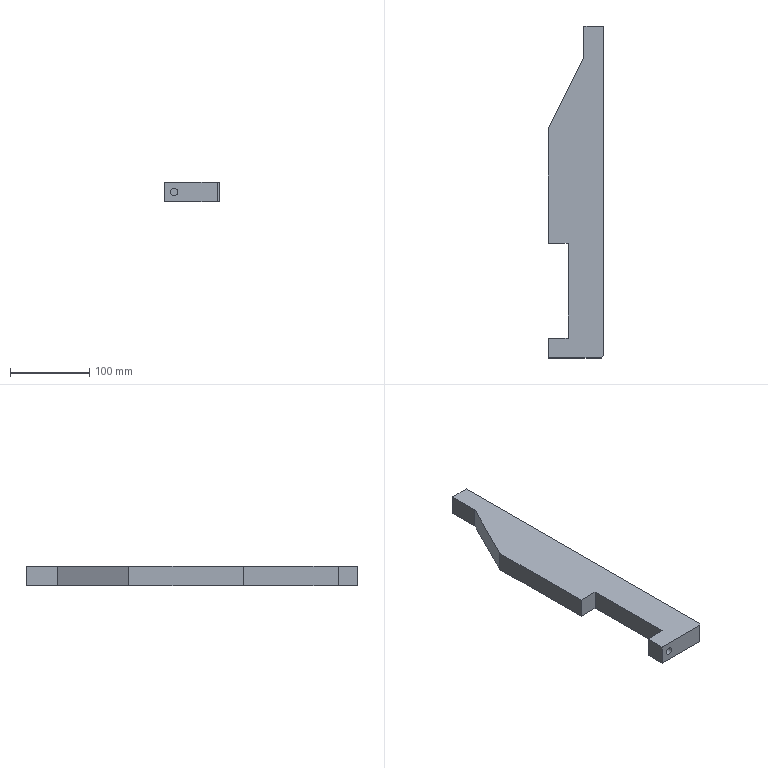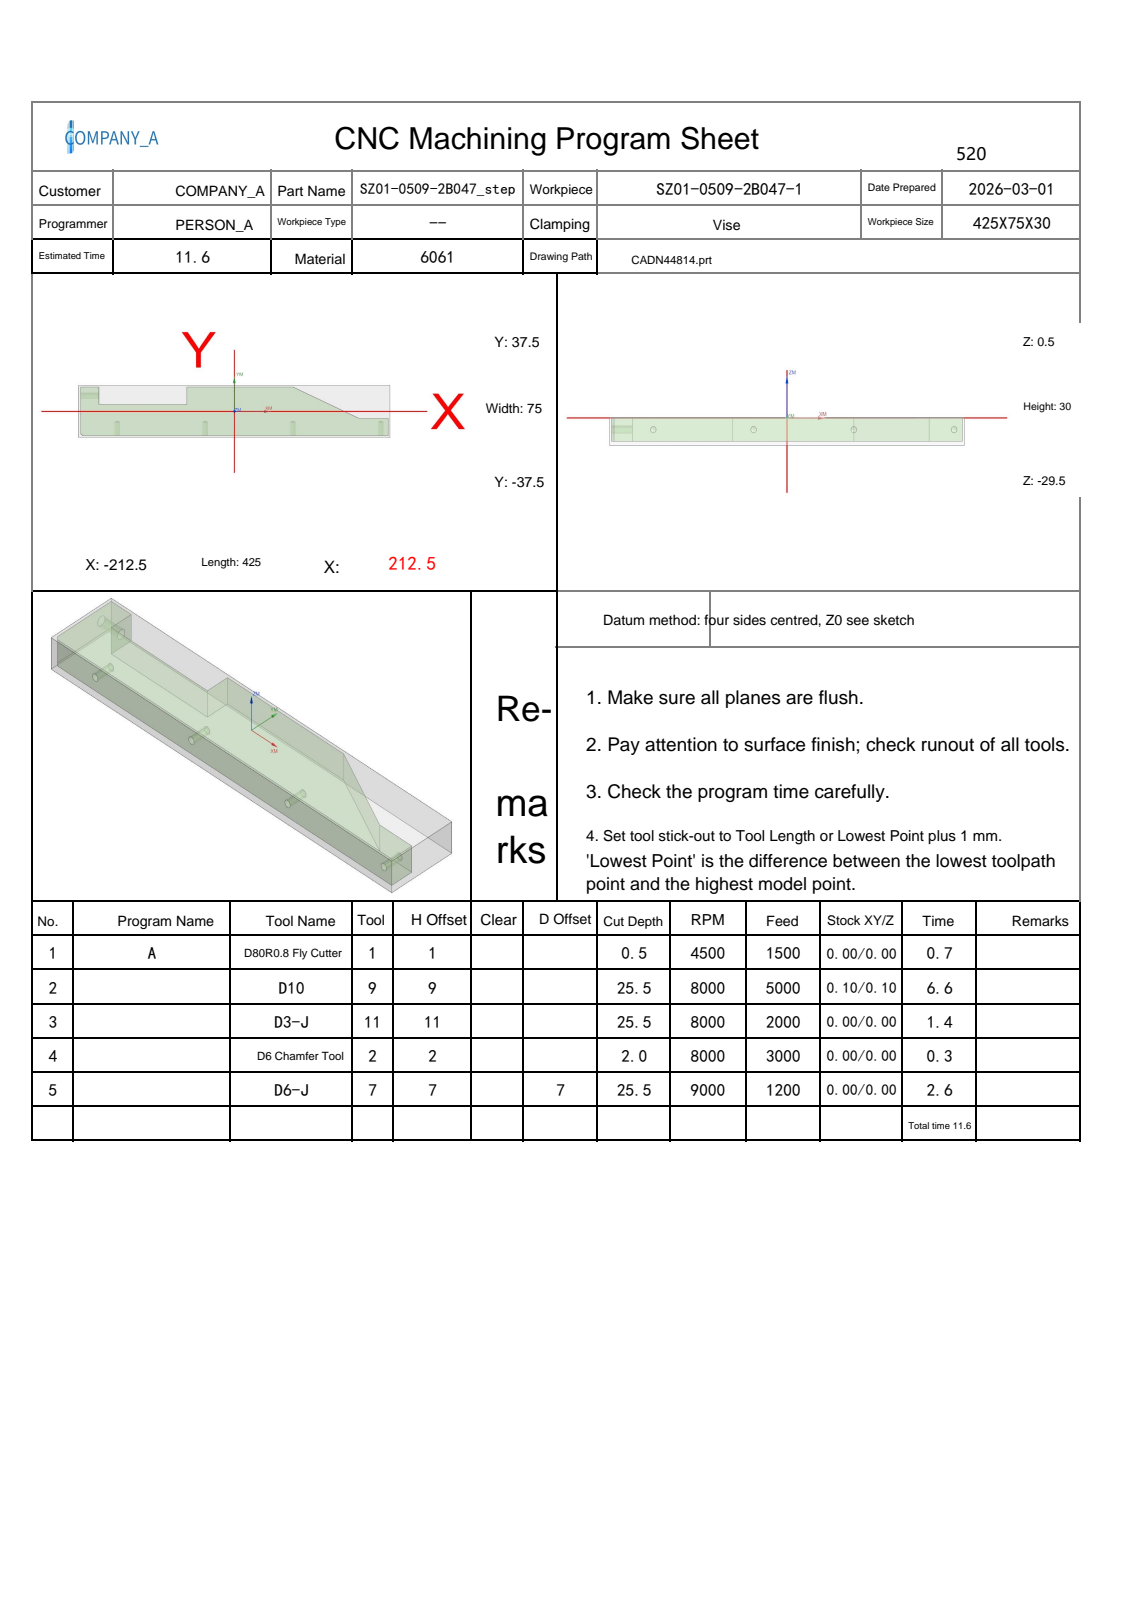NC program | NX | posted by the shop | part box 70 x 420 x 25 mm
Lines 10618 to 10764 of 10764:
N4 T02 M06
(D6 chamfer tool  D=6. R=0. H=02 ce=0.00 di=0.00)
G00 G90 G54 X1.75 Y-37.128 M03 S8000
G43 H02 Z50.
M08
Z2.099
G01 Z-1.5 F3000.
G03 X1.83 Y-36.828 I-.52 J.3
X1.53 Y-36.308 I-.6 J0.0
G01 X1.5 Y-36.3
X-207.
X-207.254 Y-36.275
X-207.497 Y-36.201
X-207.722 Y-36.081
X-207.919 Y-35.919
X-210.919 Y-32.919
X-211.081 Y-32.722
X-211.201 Y-32.497
X-211.275 Y-32.254
X-211.3 Y-32.
Y35.
G02 X-210. Y36.3 I1.3 J0.0
G01 X-185.
G02 X-183.7 Y35. I0.0 J-1.3
G01 Y11.3
X-66.3
Y35.
G02 X-65. Y36.3 I1.3 J0.0
G01 X80.
X80.299 Y36.265
X80.581 Y36.163
X170.307 Y-8.7
X210.
G02 X211.3 Y-10. I0.0 J-1.3
G01 Y-35.
G02 X210. Y-36.3 I-1.3 J0.0
G01 X1.5
X1.47 Y-36.308
G03 X1.17 Y-36.828 I.3 J-.52
X1.25 Y-37.128 I.6 J0.0
G01 Z2.099
G00 Z50.
G91 G28 Z0.0
M05
M09
G91 G28 Z0.0
M01
N5 T07 M06
(D6-J  D=6. R=0. H=07 ce=0.00 di=0.00)
G00 G90 G54 X211.017 Y-39.073 M03 S9000
G43 H07 Z50.
M08
Z-7.833
G01 Z-8.333 F1200.
G41 D07
X210.992 Y-38.875
G03 X210. Y-38. I-.992 J-.125
G01 X-207.
G02 X-209.121 Y-37.121 I0.0 J3.
G01 X-212.121 Y-34.121
G02 X-213. Y-32. I2.121 J2.121
G01 Y35.
G02 X-210. Y38. I3. J0.0
G01 X-185.
G02 X-182. Y35. I0.0 J-3.
G01 Y13.
X-68.
Y35.
G02 X-65. Y38. I3. J0.0
G01 X80.
G02 X81.342 Y37.683 I0.0 J-3.
G01 X170.708 Y-7.
X210.
G02 X213. Y-10. I0.0 J-3.
G01 Y-35.
G02 X210. Y-38. I-3. J0.0
G01 X209.5
G03 X208.5 Y-39. I0.0 J-1.
G01 G40 Y-39.2
Z-7.833
G00 Z50.
X211.017 Y-39.073
Z-16.167
G01 Z-16.667
G41 D07
X210.992 Y-38.875
G03 X210. Y-38. I-.992 J-.125
G01 X-207.
G02 X-209.121 Y-37.121 I0.0 J3.
G01 X-212.121 Y-34.121
G02 X-213. Y-32. I2.121 J2.121
G01 Y35.
G02 X-210. Y38. I3. J0.0
G01 X-185.
G02 X-182. Y35. I0.0 J-3.
G01 Y13.
X-68.
Y35.
G02 X-65. Y38. I3. J0.0
G01 X80.
G02 X81.342 Y37.683 I0.0 J-3.
G01 X170.708 Y-7.
X210.
G02 X213. Y-10. I0.0 J-3.
G01 Y-35.
G02 X210. Y-38. I-3. J0.0
G01 X209.5
G03 X208.5 Y-39. I0.0 J-1.
G01 G40 Y-39.2
Z-16.167
G00 Z50.
X211.017 Y-39.073
Z-24.5
G01 Z-25.
G41 D07
X210.992 Y-38.875
G03 X210. Y-38. I-.992 J-.125
G01 X-207.
G02 X-209.121 Y-37.121 I0.0 J3.
G01 X-212.121 Y-34.121
G02 X-213. Y-32. I2.121 J2.121
G01 Y35.
G02 X-210. Y38. I3. J0.0
G01 X-185.
G02 X-182. Y35. I0.0 J-3.
G01 Y13.
X-68.
Y35.
G02 X-65. Y38. I3. J0.0
G01 X80.
G02 X81.342 Y37.683 I0.0 J-3.
G01 X170.708 Y-7.
X210.
G02 X213. Y-10. I0.0 J-3.
G01 Y-35.
G02 X210. Y-38. I-3. J0.0
G01 X209.5
G03 X208.5 Y-39. I0.0 J-1.
G01 G40 Y-39.2
Z-24.5
G00 Z50.
M05
M09
G91 G28 Z0.0
G91 G28 Y0.0
M30
%